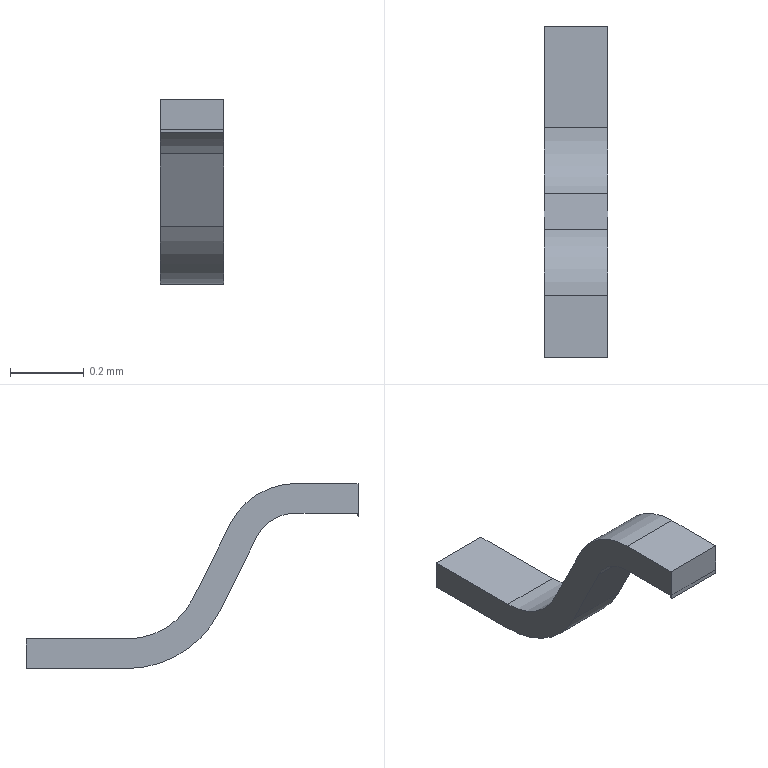Part | STEP file | RJ-USIO-V1_2-220411_5 | 1 solid | 15 faces | box 0.1708 x 0.8974 x 0.5 mm | volume 0.01511 mm3 | plane 11 | cylinder 4 | commonest cylinder face diameters 0.4 x2 0.24 x1 0.56 x1
STEP:
#1=CARTESIAN_POINT('',(0.,0.,0.));
#2=DIRECTION('',(0.,0.,1.));
#3=DIRECTION('',(1.,0.,0.));
#4=AXIS2_PLACEMENT_3D('',#1,#2,#3);
#5=CARTESIAN_POINT('',(46.936,55.937,0.3886));
#6=VERTEX_POINT('',#5);
#7=CARTESIAN_POINT('',(46.765,55.937,0.3886));
#8=VERTEX_POINT('',#7);
#9=CARTESIAN_POINT('',(46.936,55.937,0.3886));
#10=DIRECTION('',(-1.,0.,0.));
#11=VECTOR('',#10,1.);
#12=LINE('',#9,#11);
#13=CARTESIAN_POINT('',(44.809,55.758,0.3));
#14=DIRECTION('',(1.,0.,0.));
#15=DIRECTION('',(0.,0.,1.));
#16=AXIS2_PLACEMENT_3D('',#13,#14,#15);
#17=CYLINDRICAL_SURFACE('',#16,0.2);
#18=CARTESIAN_POINT('',(5.172,2.127));
#19=DIRECTION('',(0.,-1.));
#20=VECTOR('',#19,1.);
#21=LINE('',#18,#20);
#22=(GEOMETRIC_REPRESENTATION_CONTEXT(2)PARAMETRIC_REPRESENTATION_CONTEXT()REPRESENTATION_CONTEXT('',''));
#23=DEFINITIONAL_REPRESENTATION('',(#21),#22);
#24=PCURVE('',#17,#23);
#25=CARTESIAN_POINT('',(44.809,56.035,0.1914));
#26=DIRECTION('',(0.,-0.8964,-0.4432));
#27=DIRECTION('',(0.,-0.4432,0.8964));
#28=AXIS2_PLACEMENT_3D('',#25,#26,#27);
#29=PLANE('',#28);
#30=CARTESIAN_POINT('',(0.2201,-2.127));
#31=DIRECTION('',(0.,1.));
#32=VECTOR('',#31,1.);
#33=LINE('',#30,#32);
#34=(GEOMETRIC_REPRESENTATION_CONTEXT(2)PARAMETRIC_REPRESENTATION_CONTEXT()REPRESENTATION_CONTEXT('',''));
#35=DEFINITIONAL_REPRESENTATION('',(#33),#34);
#36=PCURVE('',#29,#35);
#37=SURFACE_CURVE('',#12,(#24,#36),.PCURVE_S1.);
#38=EDGE_CURVE('',#6,#8,#37,.T.);
#39=ORIENTED_EDGE('',*,*,#38,.T.);
#40=CARTESIAN_POINT('',(46.765,55.758,0.5));
#41=VERTEX_POINT('',#40);
#42=CARTESIAN_POINT('',(46.765,55.758,0.3));
#43=DIRECTION('',(-1.,0.,0.));
#44=DIRECTION('',(0.,0.,1.));
#45=AXIS2_PLACEMENT_3D('',#42,#43,#44);
#46=CIRCLE('',#45,0.2);
#47=CARTESIAN_POINT('',(6.283,1.956));
#48=DIRECTION('',(-1.,0.));
#49=VECTOR('',#48,1.);
#50=LINE('',#47,#49);
#51=(GEOMETRIC_REPRESENTATION_CONTEXT(2)PARAMETRIC_REPRESENTATION_CONTEXT()REPRESENTATION_CONTEXT('',''));
#52=DEFINITIONAL_REPRESENTATION('',(#50),#51);
#53=PCURVE('',#17,#52);
#54=CARTESIAN_POINT('',(46.765,56.487,0.5));
#55=DIRECTION('',(-1.,0.,0.));
#56=DIRECTION('',(0.,0.,-1.));
#57=AXIS2_PLACEMENT_3D('',#54,#55,#56);
#58=PLANE('',#57);
#59=CARTESIAN_POINT('',(0.2,0.7295));
#60=DIRECTION('',(-1.,0.));
#61=AXIS2_PLACEMENT_2D('',#59,#60);
#62=CIRCLE('',#61,0.2);
#63=(GEOMETRIC_REPRESENTATION_CONTEXT(2)PARAMETRIC_REPRESENTATION_CONTEXT()REPRESENTATION_CONTEXT('',''));
#64=DEFINITIONAL_REPRESENTATION('',(#62),#63);
#65=PCURVE('',#58,#64);
#66=SURFACE_CURVE('',#46,(#53,#65),.PCURVE_S1.);
#67=EDGE_CURVE('',#41,#8,#66,.T.);
#68=ORIENTED_EDGE('',*,*,#67,.F.);
#69=CARTESIAN_POINT('',(46.936,55.758,0.5));
#70=VERTEX_POINT('',#69);
#71=CARTESIAN_POINT('',(46.765,55.758,0.5));
#72=DIRECTION('',(1.,0.,0.));
#73=VECTOR('',#72,1.);
#74=LINE('',#71,#73);
#75=CARTESIAN_POINT('',(6.283,1.956));
#76=DIRECTION('',(0.,1.));
#77=VECTOR('',#76,1.);
#78=LINE('',#75,#77);
#79=(GEOMETRIC_REPRESENTATION_CONTEXT(2)PARAMETRIC_REPRESENTATION_CONTEXT()REPRESENTATION_CONTEXT('',''));
#80=DEFINITIONAL_REPRESENTATION('',(#78),#79);
#81=PCURVE('',#17,#80);
#82=CARTESIAN_POINT('',(46.936,55.59,0.5));
#83=DIRECTION('',(0.,0.,-1.));
#84=DIRECTION('',(1.,0.,0.));
#85=AXIS2_PLACEMENT_3D('',#82,#83,#84);
#86=PLANE('',#85);
#87=CARTESIAN_POINT('',(-0.1708,-0.1678));
#88=DIRECTION('',(1.,0.));
#89=VECTOR('',#88,1.);
#90=LINE('',#87,#89);
#91=(GEOMETRIC_REPRESENTATION_CONTEXT(2)PARAMETRIC_REPRESENTATION_CONTEXT()REPRESENTATION_CONTEXT('',''));
#92=DEFINITIONAL_REPRESENTATION('',(#90),#91);
#93=PCURVE('',#86,#92);
#94=SURFACE_CURVE('',#74,(#81,#93),.PCURVE_S1.);
#95=EDGE_CURVE('',#41,#70,#94,.T.);
#96=ORIENTED_EDGE('',*,*,#95,.T.);
#97=CARTESIAN_POINT('',(46.936,55.758,0.3));
#98=DIRECTION('',(1.,0.,0.));
#99=DIRECTION('',(0.,0.8964,0.4432));
#100=AXIS2_PLACEMENT_3D('',#97,#98,#99);
#101=CIRCLE('',#100,0.2);
#102=CARTESIAN_POINT('',(5.172,2.127));
#103=DIRECTION('',(1.,0.));
#104=VECTOR('',#103,1.);
#105=LINE('',#102,#104);
#106=(GEOMETRIC_REPRESENTATION_CONTEXT(2)PARAMETRIC_REPRESENTATION_CONTEXT()REPRESENTATION_CONTEXT('',''));
#107=DEFINITIONAL_REPRESENTATION('',(#105),#106);
#108=PCURVE('',#17,#107);
#109=CARTESIAN_POINT('',(46.936,56.487,0.5));
#110=DIRECTION('',(1.,0.,0.));
#111=DIRECTION('',(0.,0.,1.));
#112=AXIS2_PLACEMENT_3D('',#109,#110,#111);
#113=PLANE('',#112);
#114=CARTESIAN_POINT('',(-0.2,0.7295));
#115=DIRECTION('',(0.4432,-0.8964));
#116=AXIS2_PLACEMENT_2D('',#114,#115);
#117=CIRCLE('',#116,0.2);
#118=(GEOMETRIC_REPRESENTATION_CONTEXT(2)PARAMETRIC_REPRESENTATION_CONTEXT()REPRESENTATION_CONTEXT('',''));
#119=DEFINITIONAL_REPRESENTATION('',(#117),#118);
#120=PCURVE('',#113,#119);
#121=SURFACE_CURVE('',#101,(#108,#120),.PCURVE_S1.);
#122=EDGE_CURVE('',#6,#70,#121,.T.);
#123=ORIENTED_EDGE('',*,*,#122,.F.);
#124=EDGE_LOOP('',(#39,#68,#96,#123));
#125=FACE_BOUND('',#124,.T.);
#126=ADVANCED_FACE('',(#125),#17,.T.);
#127=CARTESIAN_POINT('',(46.936,56.487,0.08));
#128=VERTEX_POINT('',#127);
#129=CARTESIAN_POINT('',(46.936,56.214,0.08));
#130=VERTEX_POINT('',#129);
#131=CARTESIAN_POINT('',(46.936,56.487,0.08));
#132=DIRECTION('',(0.,-1.,0.));
#133=VECTOR('',#132,1.);
#134=LINE('',#131,#133);
#135=CARTESIAN_POINT('',(-0.42,0.));
#136=DIRECTION('',(0.,1.));
#137=VECTOR('',#136,1.);
#138=LINE('',#135,#137);
#139=(GEOMETRIC_REPRESENTATION_CONTEXT(2)PARAMETRIC_REPRESENTATION_CONTEXT()REPRESENTATION_CONTEXT('',''));
#140=DEFINITIONAL_REPRESENTATION('',(#138),#139);
#141=PCURVE('',#113,#140);
#142=CARTESIAN_POINT('',(44.809,56.491,0.08));
#143=DIRECTION('',(0.,0.,-1.));
#144=DIRECTION('',(1.,0.,0.));
#145=AXIS2_PLACEMENT_3D('',#142,#143,#144);
#146=PLANE('',#145);
#147=CARTESIAN_POINT('',(2.127,0.003694));
#148=DIRECTION('',(0.,1.));
#149=VECTOR('',#148,1.);
#150=LINE('',#147,#149);
#151=(GEOMETRIC_REPRESENTATION_CONTEXT(2)PARAMETRIC_REPRESENTATION_CONTEXT()REPRESENTATION_CONTEXT('',''));
#152=DEFINITIONAL_REPRESENTATION('',(#150),#151);
#153=PCURVE('',#146,#152);
#154=SURFACE_CURVE('',#134,(#141,#153),.PCURVE_S1.);
#155=EDGE_CURVE('',#128,#130,#154,.T.);
#156=ORIENTED_EDGE('',*,*,#155,.F.);
#157=CARTESIAN_POINT('',(46.936,56.487,0.));
#158=VERTEX_POINT('',#157);
#159=CARTESIAN_POINT('',(46.936,56.487,0.));
#160=DIRECTION('',(0.,0.,1.));
#161=VECTOR('',#160,1.);
#162=LINE('',#159,#161);
#163=CARTESIAN_POINT('',(-0.5,0.));
#164=DIRECTION('',(1.,0.));
#165=VECTOR('',#164,1.);
#166=LINE('',#163,#165);
#167=(GEOMETRIC_REPRESENTATION_CONTEXT(2)PARAMETRIC_REPRESENTATION_CONTEXT()REPRESENTATION_CONTEXT('',''));
#168=DEFINITIONAL_REPRESENTATION('',(#166),#167);
#169=PCURVE('',#113,#168);
#170=CARTESIAN_POINT('',(46.936,56.487,0.5));
#171=DIRECTION('',(0.,1.,0.));
#172=DIRECTION('',(0.,0.,-1.));
#173=AXIS2_PLACEMENT_3D('',#170,#171,#172);
#174=PLANE('',#173);
#175=CARTESIAN_POINT('',(0.5,0.));
#176=DIRECTION('',(-1.,0.));
#177=VECTOR('',#176,1.);
#178=LINE('',#175,#177);
#179=(GEOMETRIC_REPRESENTATION_CONTEXT(2)PARAMETRIC_REPRESENTATION_CONTEXT()REPRESENTATION_CONTEXT('',''));
#180=DEFINITIONAL_REPRESENTATION('',(#178),#179);
#181=PCURVE('',#174,#180);
#182=SURFACE_CURVE('',#162,(#169,#181),.PCURVE_S1.);
#183=EDGE_CURVE('',#158,#128,#182,.T.);
#184=ORIENTED_EDGE('',*,*,#183,.F.);
#185=CARTESIAN_POINT('',(46.936,56.214,0.));
#186=VERTEX_POINT('',#185);
#187=CARTESIAN_POINT('',(46.936,56.214,0.));
#188=DIRECTION('',(0.,1.,0.));
#189=VECTOR('',#188,1.);
#190=LINE('',#187,#189);
#191=CARTESIAN_POINT('',(-0.5,0.2734));
#192=DIRECTION('',(0.,-1.));
#193=VECTOR('',#192,1.);
#194=LINE('',#191,#193);
#195=(GEOMETRIC_REPRESENTATION_CONTEXT(2)PARAMETRIC_REPRESENTATION_CONTEXT()REPRESENTATION_CONTEXT('',''));
#196=DEFINITIONAL_REPRESENTATION('',(#194),#195);
#197=PCURVE('',#113,#196);
#198=CARTESIAN_POINT('',(46.936,55.59,0.));
#199=DIRECTION('',(0.,0.,-1.));
#200=DIRECTION('',(1.,0.,0.));
#201=AXIS2_PLACEMENT_3D('',#198,#199,#200);
#202=PLANE('',#201);
#203=CARTESIAN_POINT('',(0.,-0.6239));
#204=DIRECTION('',(0.,-1.));
#205=VECTOR('',#204,1.);
#206=LINE('',#203,#205);
#207=(GEOMETRIC_REPRESENTATION_CONTEXT(2)PARAMETRIC_REPRESENTATION_CONTEXT()REPRESENTATION_CONTEXT('',''));
#208=DEFINITIONAL_REPRESENTATION('',(#206),#207);
#209=PCURVE('',#202,#208);
#210=SURFACE_CURVE('',#190,(#197,#209),.PCURVE_S1.);
#211=EDGE_CURVE('',#186,#158,#210,.T.);
#212=ORIENTED_EDGE('',*,*,#211,.F.);
#213=CARTESIAN_POINT('',(46.936,55.963,0.1559));
#214=VERTEX_POINT('',#213);
#215=CARTESIAN_POINT('',(46.936,56.214,0.28));
#216=DIRECTION('',(1.,0.,0.));
#217=DIRECTION('',(0.,-0.8964,-0.4432));
#218=AXIS2_PLACEMENT_3D('',#215,#216,#217);
#219=CIRCLE('',#218,0.28);
#220=CARTESIAN_POINT('',(-0.22,0.2734));
#221=DIRECTION('',(-0.4432,0.8964));
#222=AXIS2_PLACEMENT_2D('',#220,#221);
#223=CIRCLE('',#222,0.28);
#224=(GEOMETRIC_REPRESENTATION_CONTEXT(2)PARAMETRIC_REPRESENTATION_CONTEXT()REPRESENTATION_CONTEXT('',''));
#225=DEFINITIONAL_REPRESENTATION('',(#223),#224);
#226=PCURVE('',#113,#225);
#227=CARTESIAN_POINT('',(44.809,56.214,0.28));
#228=DIRECTION('',(1.,0.,0.));
#229=DIRECTION('',(0.,0.,1.));
#230=AXIS2_PLACEMENT_3D('',#227,#228,#229);
#231=CYLINDRICAL_SURFACE('',#230,0.28);
#232=CARTESIAN_POINT('',(2.03,2.127));
#233=DIRECTION('',(1.,0.));
#234=VECTOR('',#233,1.);
#235=LINE('',#232,#234);
#236=(GEOMETRIC_REPRESENTATION_CONTEXT(2)PARAMETRIC_REPRESENTATION_CONTEXT()REPRESENTATION_CONTEXT('',''));
#237=DEFINITIONAL_REPRESENTATION('',(#235),#236);
#238=PCURVE('',#231,#237);
#239=SURFACE_CURVE('',#219,(#226,#238),.PCURVE_S1.);
#240=EDGE_CURVE('',#214,#186,#239,.T.);
#241=ORIENTED_EDGE('',*,*,#240,.F.);
#242=CARTESIAN_POINT('',(46.936,55.865,0.3532));
#243=VERTEX_POINT('',#242);
#244=CARTESIAN_POINT('',(46.936,55.865,0.3532));
#245=DIRECTION('',(0.,0.4432,-0.8964));
#246=VECTOR('',#245,1.);
#247=LINE('',#244,#246);
#248=CARTESIAN_POINT('',(-0.1468,0.622));
#249=DIRECTION('',(-0.8964,-0.4432));
#250=VECTOR('',#249,1.);
#251=LINE('',#248,#250);
#252=(GEOMETRIC_REPRESENTATION_CONTEXT(2)PARAMETRIC_REPRESENTATION_CONTEXT()REPRESENTATION_CONTEXT('',''));
#253=DEFINITIONAL_REPRESENTATION('',(#251),#252);
#254=PCURVE('',#113,#253);
#255=CARTESIAN_POINT('',(44.809,55.963,0.1559));
#256=DIRECTION('',(0.,0.8964,0.4432));
#257=DIRECTION('',(0.,0.4432,-0.8964));
#258=AXIS2_PLACEMENT_3D('',#255,#256,#257);
#259=PLANE('',#258);
#260=CARTESIAN_POINT('',(-0.2201,-2.127));
#261=DIRECTION('',(1.,0.));
#262=VECTOR('',#261,1.);
#263=LINE('',#260,#262);
#264=(GEOMETRIC_REPRESENTATION_CONTEXT(2)PARAMETRIC_REPRESENTATION_CONTEXT()REPRESENTATION_CONTEXT('',''));
#265=DEFINITIONAL_REPRESENTATION('',(#263),#264);
#266=PCURVE('',#259,#265);
#267=SURFACE_CURVE('',#247,(#254,#266),.PCURVE_S1.);
#268=EDGE_CURVE('',#243,#214,#267,.T.);
#269=ORIENTED_EDGE('',*,*,#268,.F.);
#270=CARTESIAN_POINT('',(46.936,55.758,0.42));
#271=VERTEX_POINT('',#270);
#272=CARTESIAN_POINT('',(46.936,55.758,0.3));
#273=DIRECTION('',(-1.,0.,0.));
#274=DIRECTION('',(0.,0.,1.));
#275=AXIS2_PLACEMENT_3D('',#272,#273,#274);
#276=CIRCLE('',#275,0.12);
#277=CARTESIAN_POINT('',(-0.08,0.7295));
#278=CARTESIAN_POINT('',(-0.08,0.5217));
#279=CARTESIAN_POINT('',(-0.26,0.6256));
#280=CARTESIAN_POINT('',(-0.44,0.7295));
#281=CARTESIAN_POINT('',(-0.26,0.8335));
#282=CARTESIAN_POINT('',(-0.08,0.9374));
#283=CARTESIAN_POINT('',(-0.08,0.7295));
#284=(BOUNDED_CURVE()B_SPLINE_CURVE(2,(#277,#278,#279,#280,#281,#282,#283),.UNSPECIFIED.,.T.,.F.)B_SPLINE_CURVE_WITH_KNOTS((1,2,2,2,2,1),(-2.094,0.,2.094,4.189,6.283,8.378),.UNSPECIFIED.)CURVE()GEOMETRIC_REPRESENTATION_ITEM()RATIONAL_B_SPLINE_CURVE((1.,0.5,1.,0.5,1.,0.5,1.))REPRESENTATION_ITEM(''));
#285=(GEOMETRIC_REPRESENTATION_CONTEXT(2)PARAMETRIC_REPRESENTATION_CONTEXT()REPRESENTATION_CONTEXT('',''));
#286=DEFINITIONAL_REPRESENTATION('',(#284),#285);
#287=PCURVE('',#113,#286);
#288=CARTESIAN_POINT('',(44.809,55.758,0.3));
#289=DIRECTION('',(1.,0.,0.));
#290=DIRECTION('',(0.,0.,1.));
#291=AXIS2_PLACEMENT_3D('',#288,#289,#290);
#292=CYLINDRICAL_SURFACE('',#291,0.12);
#293=CARTESIAN_POINT('',(6.283,2.127));
#294=DIRECTION('',(-1.,0.));
#295=VECTOR('',#294,1.);
#296=LINE('',#293,#295);
#297=(GEOMETRIC_REPRESENTATION_CONTEXT(2)PARAMETRIC_REPRESENTATION_CONTEXT()REPRESENTATION_CONTEXT('',''));
#298=DEFINITIONAL_REPRESENTATION('',(#296),#297);
#299=PCURVE('',#292,#298);
#300=SURFACE_CURVE('',#276,(#287,#299),.PCURVE_S1.);
#301=EDGE_CURVE('',#271,#243,#300,.T.);
#302=ORIENTED_EDGE('',*,*,#301,.F.);
#303=CARTESIAN_POINT('',(46.936,55.591,0.42));
#304=VERTEX_POINT('',#303);
#305=CARTESIAN_POINT('',(46.936,55.591,0.42));
#306=DIRECTION('',(0.,1.,0.));
#307=VECTOR('',#306,1.);
#308=LINE('',#305,#307);
#309=CARTESIAN_POINT('',(-0.08,0.8961));
#310=DIRECTION('',(0.,-1.));
#311=VECTOR('',#310,1.);
#312=LINE('',#309,#311);
#313=(GEOMETRIC_REPRESENTATION_CONTEXT(2)PARAMETRIC_REPRESENTATION_CONTEXT()REPRESENTATION_CONTEXT('',''));
#314=DEFINITIONAL_REPRESENTATION('',(#312),#313);
#315=PCURVE('',#113,#314);
#316=CARTESIAN_POINT('',(44.809,55.758,0.42));
#317=DIRECTION('',(0.,0.,1.));
#318=DIRECTION('',(-1.,0.,0.));
#319=AXIS2_PLACEMENT_3D('',#316,#317,#318);
#320=PLANE('',#319);
#321=CARTESIAN_POINT('',(-2.127,0.1665));
#322=DIRECTION('',(0.,-1.));
#323=VECTOR('',#322,1.);
#324=LINE('',#321,#323);
#325=(GEOMETRIC_REPRESENTATION_CONTEXT(2)PARAMETRIC_REPRESENTATION_CONTEXT()REPRESENTATION_CONTEXT('',''));
#326=DEFINITIONAL_REPRESENTATION('',(#324),#325);
#327=PCURVE('',#320,#326);
#328=SURFACE_CURVE('',#308,(#315,#327),.PCURVE_S1.);
#329=EDGE_CURVE('',#304,#271,#328,.T.);
#330=ORIENTED_EDGE('',*,*,#329,.F.);
#331=CARTESIAN_POINT('',(46.936,55.59,0.4096));
#332=VERTEX_POINT('',#331);
#333=CARTESIAN_POINT('',(46.936,55.59,0.4096));
#334=DIRECTION('',(0.,0.1219,0.9925));
#335=VECTOR('',#334,1.);
#336=LINE('',#333,#335);
#337=CARTESIAN_POINT('',(-0.09045,0.8974));
#338=DIRECTION('',(0.9925,-0.1219));
#339=VECTOR('',#338,1.);
#340=LINE('',#337,#339);
#341=(GEOMETRIC_REPRESENTATION_CONTEXT(2)PARAMETRIC_REPRESENTATION_CONTEXT()REPRESENTATION_CONTEXT('',''));
#342=DEFINITIONAL_REPRESENTATION('',(#340),#341);
#343=PCURVE('',#113,#342);
#344=CARTESIAN_POINT('',(44.809,55.591,0.42));
#345=DIRECTION('',(0.,-0.9925,0.1219));
#346=DIRECTION('',(0.,0.1219,0.9925));
#347=AXIS2_PLACEMENT_3D('',#344,#345,#346);
#348=PLANE('',#347);
#349=CARTESIAN_POINT('',(-0.01053,-2.127));
#350=DIRECTION('',(1.,0.));
#351=VECTOR('',#350,1.);
#352=LINE('',#349,#351);
#353=(GEOMETRIC_REPRESENTATION_CONTEXT(2)PARAMETRIC_REPRESENTATION_CONTEXT()REPRESENTATION_CONTEXT('',''));
#354=DEFINITIONAL_REPRESENTATION('',(#352),#353);
#355=PCURVE('',#348,#354);
#356=SURFACE_CURVE('',#336,(#343,#355),.PCURVE_S1.);
#357=EDGE_CURVE('',#332,#304,#356,.T.);
#358=ORIENTED_EDGE('',*,*,#357,.F.);
#359=CARTESIAN_POINT('',(46.936,55.59,0.5));
#360=VERTEX_POINT('',#359);
#361=CARTESIAN_POINT('',(46.936,55.59,0.4096));
#362=DIRECTION('',(0.,0.,1.));
#363=VECTOR('',#362,1.);
#364=LINE('',#361,#363);
#365=CARTESIAN_POINT('',(-0.09045,0.8974));
#366=DIRECTION('',(1.,0.));
#367=VECTOR('',#366,1.);
#368=LINE('',#365,#367);
#369=(GEOMETRIC_REPRESENTATION_CONTEXT(2)PARAMETRIC_REPRESENTATION_CONTEXT()REPRESENTATION_CONTEXT('',''));
#370=DEFINITIONAL_REPRESENTATION('',(#368),#369);
#371=PCURVE('',#113,#370);
#372=CARTESIAN_POINT('',(46.936,55.59,0.5));
#373=DIRECTION('',(0.,-1.,0.));
#374=DIRECTION('',(0.,0.,1.));
#375=AXIS2_PLACEMENT_3D('',#372,#373,#374);
#376=PLANE('',#375);
#377=CARTESIAN_POINT('',(-0.09045,0.));
#378=DIRECTION('',(1.,0.));
#379=VECTOR('',#378,1.);
#380=LINE('',#377,#379);
#381=(GEOMETRIC_REPRESENTATION_CONTEXT(2)PARAMETRIC_REPRESENTATION_CONTEXT()REPRESENTATION_CONTEXT('',''));
#382=DEFINITIONAL_REPRESENTATION('',(#380),#381);
#383=PCURVE('',#376,#382);
#384=SURFACE_CURVE('',#364,(#371,#383),.PCURVE_S1.);
#385=EDGE_CURVE('',#332,#360,#384,.T.);
#386=ORIENTED_EDGE('',*,*,#385,.T.);
#387=CARTESIAN_POINT('',(46.936,55.59,0.5));
#388=DIRECTION('',(0.,1.,0.));
#389=VECTOR('',#388,1.);
#390=LINE('',#387,#389);
#391=CARTESIAN_POINT('',(0.,0.8974));
#392=DIRECTION('',(0.,-1.));
#393=VECTOR('',#392,1.);
#394=LINE('',#391,#393);
#395=(GEOMETRIC_REPRESENTATION_CONTEXT(2)PARAMETRIC_REPRESENTATION_CONTEXT()REPRESENTATION_CONTEXT('',''));
#396=DEFINITIONAL_REPRESENTATION('',(#394),#395);
#397=PCURVE('',#113,#396);
#398=CARTESIAN_POINT('',(0.,0.));
#399=DIRECTION('',(0.,-1.));
#400=VECTOR('',#399,1.);
#401=LINE('',#398,#400);
#402=(GEOMETRIC_REPRESENTATION_CONTEXT(2)PARAMETRIC_REPRESENTATION_CONTEXT()REPRESENTATION_CONTEXT('',''));
#403=DEFINITIONAL_REPRESENTATION('',(#401),#402);
#404=PCURVE('',#86,#403);
#405=SURFACE_CURVE('',#390,(#397,#404),.PCURVE_S1.);
#406=EDGE_CURVE('',#360,#70,#405,.T.);
#407=ORIENTED_EDGE('',*,*,#406,.T.);
#408=ORIENTED_EDGE('',*,*,#122,.F.);
#409=CARTESIAN_POINT('',(46.936,56.035,0.1914));
#410=VERTEX_POINT('',#409);
#411=CARTESIAN_POINT('',(46.936,56.035,0.1914));
#412=DIRECTION('',(0.,-0.4432,0.8964));
#413=VECTOR('',#412,1.);
#414=LINE('',#411,#413);
#415=CARTESIAN_POINT('',(-0.3086,0.4527));
#416=DIRECTION('',(0.8964,0.4432));
#417=VECTOR('',#416,1.);
#418=LINE('',#415,#417);
#419=(GEOMETRIC_REPRESENTATION_CONTEXT(2)PARAMETRIC_REPRESENTATION_CONTEXT()REPRESENTATION_CONTEXT('',''));
#420=DEFINITIONAL_REPRESENTATION('',(#418),#419);
#421=PCURVE('',#113,#420);
#422=CARTESIAN_POINT('',(0.,-2.127));
#423=DIRECTION('',(1.,0.));
#424=VECTOR('',#423,1.);
#425=LINE('',#422,#424);
#426=(GEOMETRIC_REPRESENTATION_CONTEXT(2)PARAMETRIC_REPRESENTATION_CONTEXT()REPRESENTATION_CONTEXT('',''));
#427=DEFINITIONAL_REPRESENTATION('',(#425),#426);
#428=PCURVE('',#29,#427);
#429=SURFACE_CURVE('',#414,(#421,#428),.PCURVE_S1.);
#430=EDGE_CURVE('',#410,#6,#429,.T.);
#431=ORIENTED_EDGE('',*,*,#430,.F.);
#432=CARTESIAN_POINT('',(46.936,56.214,0.28));
#433=DIRECTION('',(-1.,0.,0.));
#434=DIRECTION('',(0.,0.,-1.));
#435=AXIS2_PLACEMENT_3D('',#432,#433,#434);
#436=CIRCLE('',#435,0.2);
#437=CARTESIAN_POINT('',(-0.42,0.2734));
#438=CARTESIAN_POINT('',(-0.42,0.6198));
#439=CARTESIAN_POINT('',(-0.12,0.4466));
#440=CARTESIAN_POINT('',(0.18,0.2734));
#441=CARTESIAN_POINT('',(-0.12,0.1002));
#442=CARTESIAN_POINT('',(-0.42,-0.07299));
#443=CARTESIAN_POINT('',(-0.42,0.2734));
#444=(BOUNDED_CURVE()B_SPLINE_CURVE(2,(#437,#438,#439,#440,#441,#442,#443),.UNSPECIFIED.,.T.,.F.)B_SPLINE_CURVE_WITH_KNOTS((1,2,2,2,2,1),(-2.094,0.,2.094,4.189,6.283,8.378),.UNSPECIFIED.)CURVE()GEOMETRIC_REPRESENTATION_ITEM()RATIONAL_B_SPLINE_CURVE((1.,0.5,1.,0.5,1.,0.5,1.))REPRESENTATION_ITEM(''));
#445=(GEOMETRIC_REPRESENTATION_CONTEXT(2)PARAMETRIC_REPRESENTATION_CONTEXT()REPRESENTATION_CONTEXT('',''));
#446=DEFINITIONAL_REPRESENTATION('',(#444),#445);
#447=PCURVE('',#113,#446);
#448=CARTESIAN_POINT('',(44.809,56.214,0.28));
#449=DIRECTION('',(1.,0.,0.));
#450=DIRECTION('',(0.,0.,1.));
#451=AXIS2_PLACEMENT_3D('',#448,#449,#450);
#452=CYLINDRICAL_SURFACE('',#451,0.2);
#453=CARTESIAN_POINT('',(3.142,2.127));
#454=DIRECTION('',(-1.,0.));
#455=VECTOR('',#454,1.);
#456=LINE('',#453,#455);
#457=(GEOMETRIC_REPRESENTATION_CONTEXT(2)PARAMETRIC_REPRESENTATION_CONTEXT()REPRESENTATION_CONTEXT('',''));
#458=DEFINITIONAL_REPRESENTATION('',(#456),#457);
#459=PCURVE('',#452,#458);
#460=SURFACE_CURVE('',#436,(#447,#459),.PCURVE_S1.);
#461=EDGE_CURVE('',#130,#410,#460,.T.);
#462=ORIENTED_EDGE('',*,*,#461,.F.);
#463=EDGE_LOOP('',(#156,#184,#212,#241,#269,#302,#330,#358,#386,#407,#408,#431,#462));
#464=FACE_BOUND('',#463,.F.);
#465=ADVANCED_FACE('',(#464),#113,.T.);
#466=ORIENTED_EDGE('',*,*,#155,.T.);
#467=CARTESIAN_POINT('',(46.765,56.214,0.08));
#468=VERTEX_POINT('',#467);
#469=CARTESIAN_POINT('',(46.936,56.214,0.08));
#470=DIRECTION('',(-1.,0.,0.));
#471=VECTOR('',#470,1.);
#472=LINE('',#469,#471);
#473=CARTESIAN_POINT('',(2.127,0.2771));
#474=DIRECTION('',(-1.,0.));
#475=VECTOR('',#474,1.);
#476=LINE('',#473,#475);
#477=(GEOMETRIC_REPRESENTATION_CONTEXT(2)PARAMETRIC_REPRESENTATION_CONTEXT()REPRESENTATION_CONTEXT('',''));
#478=DEFINITIONAL_REPRESENTATION('',(#476),#477);
#479=PCURVE('',#146,#478);
#480=CARTESIAN_POINT('',(3.142,2.127));
#481=DIRECTION('',(0.,-1.));
#482=VECTOR('',#481,1.);
#483=LINE('',#480,#482);
#484=(GEOMETRIC_REPRESENTATION_CONTEXT(2)PARAMETRIC_REPRESENTATION_CONTEXT()REPRESENTATION_CONTEXT('',''));
#485=DEFINITIONAL_REPRESENTATION('',(#483),#484);
#486=PCURVE('',#452,#485);
#487=SURFACE_CURVE('',#472,(#479,#486),.PCURVE_S1.);
#488=EDGE_CURVE('',#130,#468,#487,.T.);
#489=ORIENTED_EDGE('',*,*,#488,.T.);
#490=CARTESIAN_POINT('',(46.765,56.487,0.08));
#491=VERTEX_POINT('',#490);
#492=CARTESIAN_POINT('',(46.765,56.214,0.08));
#493=DIRECTION('',(0.,1.,0.));
#494=VECTOR('',#493,1.);
#495=LINE('',#492,#494);
#496=CARTESIAN_POINT('',(1.956,0.2771));
#497=DIRECTION('',(0.,-1.));
#498=VECTOR('',#497,1.);
#499=LINE('',#496,#498);
#500=(GEOMETRIC_REPRESENTATION_CONTEXT(2)PARAMETRIC_REPRESENTATION_CONTEXT()REPRESENTATION_CONTEXT('',''));
#501=DEFINITIONAL_REPRESENTATION('',(#499),#500);
#502=PCURVE('',#146,#501);
#503=CARTESIAN_POINT('',(0.42,0.2734));
#504=DIRECTION('',(0.,-1.));
#505=VECTOR('',#504,1.);
#506=LINE('',#503,#505);
#507=(GEOMETRIC_REPRESENTATION_CONTEXT(2)PARAMETRIC_REPRESENTATION_CONTEXT()REPRESENTATION_CONTEXT('',''));
#508=DEFINITIONAL_REPRESENTATION('',(#506),#507);
#509=PCURVE('',#58,#508);
#510=SURFACE_CURVE('',#495,(#502,#509),.PCURVE_S1.);
#511=EDGE_CURVE('',#468,#491,#510,.T.);
#512=ORIENTED_EDGE('',*,*,#511,.T.);
#513=CARTESIAN_POINT('',(46.765,56.487,0.08));
#514=DIRECTION('',(1.,0.,0.));
#515=VECTOR('',#514,1.);
#516=LINE('',#513,#515);
#517=CARTESIAN_POINT('',(1.956,0.003694));
#518=DIRECTION('',(1.,0.));
#519=VECTOR('',#518,1.);
#520=LINE('',#517,#519);
#521=(GEOMETRIC_REPRESENTATION_CONTEXT(2)PARAMETRIC_REPRESENTATION_CONTEXT()REPRESENTATION_CONTEXT('',''));
#522=DEFINITIONAL_REPRESENTATION('',(#520),#521);
#523=PCURVE('',#146,#522);
#524=CARTESIAN_POINT('',(0.42,0.1708));
#525=DIRECTION('',(0.,-1.));
#526=VECTOR('',#525,1.);
#527=LINE('',#524,#526);
#528=(GEOMETRIC_REPRESENTATION_CONTEXT(2)PARAMETRIC_REPRESENTATION_CONTEXT()REPRESENTATION_CONTEXT('',''));
#529=DEFINITIONAL_REPRESENTATION('',(#527),#528);
#530=PCURVE('',#174,#529);
#531=SURFACE_CURVE('',#516,(#523,#530),.PCURVE_S1.);
#532=EDGE_CURVE('',#491,#128,#531,.T.);
#533=ORIENTED_EDGE('',*,*,#532,.T.);
#534=EDGE_LOOP('',(#466,#489,#512,#533));
#535=FACE_BOUND('',#534,.F.);
#536=ADVANCED_FACE('',(#535),#146,.F.);
#537=ORIENTED_EDGE('',*,*,#461,.T.);
#538=CARTESIAN_POINT('',(46.765,56.035,0.1914));
#539=VERTEX_POINT('',#538);
#540=CARTESIAN_POINT('',(46.765,56.035,0.1914));
#541=DIRECTION('',(1.,0.,0.));
#542=VECTOR('',#541,1.);
#543=LINE('',#540,#542);
#544=CARTESIAN_POINT('',(2.03,1.956));
#545=DIRECTION('',(0.,1.));
#546=VECTOR('',#545,1.);
#547=LINE('',#544,#546);
#548=(GEOMETRIC_REPRESENTATION_CONTEXT(2)PARAMETRIC_REPRESENTATION_CONTEXT()REPRESENTATION_CONTEXT('',''));
#549=DEFINITIONAL_REPRESENTATION('',(#547),#548);
#550=PCURVE('',#452,#549);
#551=CARTESIAN_POINT('',(0.,-1.956));
#552=DIRECTION('',(0.,-1.));
#553=VECTOR('',#552,1.);
#554=LINE('',#551,#553);
#555=(GEOMETRIC_REPRESENTATION_CONTEXT(2)PARAMETRIC_REPRESENTATION_CONTEXT()REPRESENTATION_CONTEXT('',''));
#556=DEFINITIONAL_REPRESENTATION('',(#554),#555);
#557=PCURVE('',#29,#556);
#558=SURFACE_CURVE('',#543,(#550,#557),.PCURVE_S1.);
#559=EDGE_CURVE('',#539,#410,#558,.T.);
#560=ORIENTED_EDGE('',*,*,#559,.F.);
#561=CARTESIAN_POINT('',(46.765,56.214,0.28));
#562=DIRECTION('',(1.,0.,0.));
#563=DIRECTION('',(0.,-0.8964,-0.4432));
#564=AXIS2_PLACEMENT_3D('',#561,#562,#563);
#565=CIRCLE('',#564,0.2);
#566=CARTESIAN_POINT('',(2.03,1.956));
#567=DIRECTION('',(1.,0.));
#568=VECTOR('',#567,1.);
#569=LINE('',#566,#568);
#570=(GEOMETRIC_REPRESENTATION_CONTEXT(2)PARAMETRIC_REPRESENTATION_CONTEXT()REPRESENTATION_CONTEXT('',''));
#571=DEFINITIONAL_REPRESENTATION('',(#569),#570);
#572=PCURVE('',#452,#571);
#573=CARTESIAN_POINT('',(0.3086,0.4527));
#574=CARTESIAN_POINT('',(0.6192,0.2992));
#575=CARTESIAN_POINT('',(0.3309,0.107));
#576=CARTESIAN_POINT('',(0.0427,-0.08514));
#577=CARTESIAN_POINT('',(0.02041,0.2606));
#578=CARTESIAN_POINT('',(-0.001873,0.6062));
#579=CARTESIAN_POINT('',(0.3086,0.4527));
#580=(BOUNDED_CURVE()B_SPLINE_CURVE(2,(#573,#574,#575,#576,#577,#578,#579),.UNSPECIFIED.,.T.,.F.)B_SPLINE_CURVE_WITH_KNOTS((1,2,2,2,2,1),(-2.094,0.,2.094,4.189,6.283,8.378),.UNSPECIFIED.)CURVE()GEOMETRIC_REPRESENTATION_ITEM()RATIONAL_B_SPLINE_CURVE((1.,0.5,1.,0.5,1.,0.5,1.))REPRESENTATION_ITEM(''));
#581=(GEOMETRIC_REPRESENTATION_CONTEXT(2)PARAMETRIC_REPRESENTATION_CONTEXT()REPRESENTATION_CONTEXT('',''));
#582=DEFINITIONAL_REPRESENTATION('',(#580),#581);
#583=PCURVE('',#58,#582);
#584=SURFACE_CURVE('',#565,(#572,#583),.PCURVE_S1.);
#585=EDGE_CURVE('',#539,#468,#584,.T.);
#586=ORIENTED_EDGE('',*,*,#585,.T.);
#587=ORIENTED_EDGE('',*,*,#488,.F.);
#588=EDGE_LOOP('',(#537,#560,#586,#587));
#589=FACE_BOUND('',#588,.F.);
#590=ADVANCED_FACE('',(#589),#452,.F.);
#591=ORIENTED_EDGE('',*,*,#430,.T.);
#592=ORIENTED_EDGE('',*,*,#38,.T.);
#593=CARTESIAN_POINT('',(46.765,55.937,0.3886));
#594=DIRECTION('',(0.,0.4432,-0.8964));
#595=VECTOR('',#594,1.);
#596=LINE('',#593,#595);
#597=CARTESIAN_POINT('',(0.2201,-1.956));
#598=DIRECTION('',(-1.,0.));
#599=VECTOR('',#598,1.);
#600=LINE('',#597,#599);
#601=(GEOMETRIC_REPRESENTATION_CONTEXT(2)PARAMETRIC_REPRESENTATION_CONTEXT()REPRESENTATION_CONTEXT('',''));
#602=DEFINITIONAL_REPRESENTATION('',(#600),#601);
#603=PCURVE('',#29,#602);
#604=CARTESIAN_POINT('',(0.1114,0.5503));
#605=DIRECTION('',(0.8964,-0.4432));
#606=VECTOR('',#605,1.);
#607=LINE('',#604,#606);
#608=(GEOMETRIC_REPRESENTATION_CONTEXT(2)PARAMETRIC_REPRESENTATION_CONTEXT()REPRESENTATION_CONTEXT('',''));
#609=DEFINITIONAL_REPRESENTATION('',(#607),#608);
#610=PCURVE('',#58,#609);
#611=SURFACE_CURVE('',#596,(#603,#610),.PCURVE_S1.);
#612=EDGE_CURVE('',#8,#539,#611,.T.);
#613=ORIENTED_EDGE('',*,*,#612,.T.);
#614=ORIENTED_EDGE('',*,*,#559,.T.);
#615=EDGE_LOOP('',(#591,#592,#613,#614));
#616=FACE_BOUND('',#615,.F.);
#617=ADVANCED_FACE('',(#616),#29,.F.);
#618=ORIENTED_EDGE('',*,*,#511,.F.);
#619=ORIENTED_EDGE('',*,*,#585,.F.);
#620=ORIENTED_EDGE('',*,*,#612,.F.);
#621=ORIENTED_EDGE('',*,*,#67,.F.);
#622=CARTESIAN_POINT('',(46.765,55.59,0.5));
#623=VERTEX_POINT('',#622);
#624=CARTESIAN_POINT('',(46.765,55.758,0.5));
#625=DIRECTION('',(0.,-1.,0.));
#626=VECTOR('',#625,1.);
#627=LINE('',#624,#626);
#628=CARTESIAN_POINT('',(0.,0.7295));
#629=DIRECTION('',(0.,1.));
#630=VECTOR('',#629,1.);
#631=LINE('',#628,#630);
#632=(GEOMETRIC_REPRESENTATION_CONTEXT(2)PARAMETRIC_REPRESENTATION_CONTEXT()REPRESENTATION_CONTEXT('',''));
#633=DEFINITIONAL_REPRESENTATION('',(#631),#632);
#634=PCURVE('',#58,#633);
#635=CARTESIAN_POINT('',(-0.1708,-0.1678));
#636=DIRECTION('',(0.,1.));
#637=VECTOR('',#636,1.);
#638=LINE('',#635,#637);
#639=(GEOMETRIC_REPRESENTATION_CONTEXT(2)PARAMETRIC_REPRESENTATION_CONTEXT()REPRESENTATION_CONTEXT('',''));
#640=DEFINITIONAL_REPRESENTATION('',(#638),#639);
#641=PCURVE('',#86,#640);
#642=SURFACE_CURVE('',#627,(#634,#641),.PCURVE_S1.);
#643=EDGE_CURVE('',#41,#623,#642,.T.);
#644=ORIENTED_EDGE('',*,*,#643,.T.);
#645=CARTESIAN_POINT('',(46.765,55.59,0.4096));
#646=VERTEX_POINT('',#645);
#647=CARTESIAN_POINT('',(46.765,55.59,0.4096));
#648=DIRECTION('',(0.,0.,1.));
#649=VECTOR('',#648,1.);
#650=LINE('',#647,#649);
#651=CARTESIAN_POINT('',(0.09045,0.8974));
#652=DIRECTION('',(-1.,0.));
#653=VECTOR('',#652,1.);
#654=LINE('',#651,#653);
#655=(GEOMETRIC_REPRESENTATION_CONTEXT(2)PARAMETRIC_REPRESENTATION_CONTEXT()REPRESENTATION_CONTEXT('',''));
#656=DEFINITIONAL_REPRESENTATION('',(#654),#655);
#657=PCURVE('',#58,#656);
#658=CARTESIAN_POINT('',(-0.09045,0.1708));
#659=DIRECTION('',(1.,0.));
#660=VECTOR('',#659,1.);
#661=LINE('',#658,#660);
#662=(GEOMETRIC_REPRESENTATION_CONTEXT(2)PARAMETRIC_REPRESENTATION_CONTEXT()REPRESENTATION_CONTEXT('',''));
#663=DEFINITIONAL_REPRESENTATION('',(#661),#662);
#664=PCURVE('',#376,#663);
#665=SURFACE_CURVE('',#650,(#657,#664),.PCURVE_S1.);
#666=EDGE_CURVE('',#646,#623,#665,.T.);
#667=ORIENTED_EDGE('',*,*,#666,.F.);
#668=CARTESIAN_POINT('',(46.765,55.591,0.42));
#669=VERTEX_POINT('',#668);
#670=CARTESIAN_POINT('',(46.765,55.591,0.42));
#671=DIRECTION('',(0.,-0.1219,-0.9925));
#672=VECTOR('',#671,1.);
#673=LINE('',#670,#672);
#674=CARTESIAN_POINT('',(0.08,0.8961));
#675=DIRECTION('',(0.9925,0.1219));
#676=VECTOR('',#675,1.);
#677=LINE('',#674,#676);
#678=(GEOMETRIC_REPRESENTATION_CONTEXT(2)PARAMETRIC_REPRESENTATION_CONTEXT()REPRESENTATION_CONTEXT('',''));
#679=DEFINITIONAL_REPRESENTATION('',(#677),#678);
#680=PCURVE('',#58,#679);
#681=CARTESIAN_POINT('',(0.,-1.956));
#682=DIRECTION('',(-1.,0.));
#683=VECTOR('',#682,1.);
#684=LINE('',#681,#683);
#685=(GEOMETRIC_REPRESENTATION_CONTEXT(2)PARAMETRIC_REPRESENTATION_CONTEXT()REPRESENTATION_CONTEXT('',''));
#686=DEFINITIONAL_REPRESENTATION('',(#684),#685);
#687=PCURVE('',#348,#686);
#688=SURFACE_CURVE('',#673,(#680,#687),.PCURVE_S1.);
#689=EDGE_CURVE('',#669,#646,#688,.T.);
#690=ORIENTED_EDGE('',*,*,#689,.F.);
#691=CARTESIAN_POINT('',(46.765,55.758,0.42));
#692=VERTEX_POINT('',#691);
#693=CARTESIAN_POINT('',(46.765,55.758,0.42));
#694=DIRECTION('',(0.,-1.,0.));
#695=VECTOR('',#694,1.);
#696=LINE('',#693,#695);
#697=CARTESIAN_POINT('',(0.08,0.7295));
#698=DIRECTION('',(0.,1.));
#699=VECTOR('',#698,1.);
#700=LINE('',#697,#699);
#701=(GEOMETRIC_REPRESENTATION_CONTEXT(2)PARAMETRIC_REPRESENTATION_CONTEXT()REPRESENTATION_CONTEXT('',''));
#702=DEFINITIONAL_REPRESENTATION('',(#700),#701);
#703=PCURVE('',#58,#702);
#704=CARTESIAN_POINT('',(-1.956,0.));
#705=DIRECTION('',(0.,1.));
#706=VECTOR('',#705,1.);
#707=LINE('',#704,#706);
#708=(GEOMETRIC_REPRESENTATION_CONTEXT(2)PARAMETRIC_REPRESENTATION_CONTEXT()REPRESENTATION_CONTEXT('',''));
#709=DEFINITIONAL_REPRESENTATION('',(#707),#708);
#710=PCURVE('',#320,#709);
#711=SURFACE_CURVE('',#696,(#703,#710),.PCURVE_S1.);
#712=EDGE_CURVE('',#692,#669,#711,.T.);
#713=ORIENTED_EDGE('',*,*,#712,.F.);
#714=CARTESIAN_POINT('',(46.765,55.865,0.3532));
#715=VERTEX_POINT('',#714);
#716=CARTESIAN_POINT('',(46.765,55.758,0.3));
#717=DIRECTION('',(1.,0.,0.));
#718=DIRECTION('',(0.,0.8964,0.4432));
#719=AXIS2_PLACEMENT_3D('',#716,#717,#718);
#720=CIRCLE('',#719,0.12);
#721=CARTESIAN_POINT('',(0.1468,0.622));
#722=CARTESIAN_POINT('',(-0.0395,0.7141));
#723=CARTESIAN_POINT('',(0.1334,0.8294));
#724=CARTESIAN_POINT('',(0.3064,0.9447));
#725=CARTESIAN_POINT('',(0.3198,0.7373));
#726=CARTESIAN_POINT('',(0.3331,0.5298));
#727=CARTESIAN_POINT('',(0.1468,0.622));
#728=(BOUNDED_CURVE()B_SPLINE_CURVE(2,(#721,#722,#723,#724,#725,#726,#727),.UNSPECIFIED.,.T.,.F.)B_SPLINE_CURVE_WITH_KNOTS((1,2,2,2,2,1),(-2.094,0.,2.094,4.189,6.283,8.378),.UNSPECIFIED.)CURVE()GEOMETRIC_REPRESENTATION_ITEM()RATIONAL_B_SPLINE_CURVE((1.,0.5,1.,0.5,1.,0.5,1.))REPRESENTATION_ITEM(''));
#729=(GEOMETRIC_REPRESENTATION_CONTEXT(2)PARAMETRIC_REPRESENTATION_CONTEXT()REPRESENTATION_CONTEXT('',''));
#730=DEFINITIONAL_REPRESENTATION('',(#728),#729);
#731=PCURVE('',#58,#730);
#732=CARTESIAN_POINT('',(5.172,1.956));
#733=DIRECTION('',(1.,0.));
#734=VECTOR('',#733,1.);
#735=LINE('',#732,#734);
#736=(GEOMETRIC_REPRESENTATION_CONTEXT(2)PARAMETRIC_REPRESENTATION_CONTEXT()REPRESENTATION_CONTEXT('',''));
#737=DEFINITIONAL_REPRESENTATION('',(#735),#736);
#738=PCURVE('',#292,#737);
#739=SURFACE_CURVE('',#720,(#731,#738),.PCURVE_S1.);
#740=EDGE_CURVE('',#715,#692,#739,.T.);
#741=ORIENTED_EDGE('',*,*,#740,.F.);
#742=CARTESIAN_POINT('',(46.765,55.963,0.1559));
#743=VERTEX_POINT('',#742);
#744=CARTESIAN_POINT('',(46.765,55.963,0.1559));
#745=DIRECTION('',(0.,-0.4432,0.8964));
#746=VECTOR('',#745,1.);
#747=LINE('',#744,#746);
#748=CARTESIAN_POINT('',(0.3441,0.5244));
#749=DIRECTION('',(-0.8964,0.4432));
#750=VECTOR('',#749,1.);
#751=LINE('',#748,#750);
#752=(GEOMETRIC_REPRESENTATION_CONTEXT(2)PARAMETRIC_REPRESENTATION_CONTEXT()REPRESENTATION_CONTEXT('',''));
#753=DEFINITIONAL_REPRESENTATION('',(#751),#752);
#754=PCURVE('',#58,#753);
#755=CARTESIAN_POINT('',(0.,-1.956));
#756=DIRECTION('',(-1.,0.));
#757=VECTOR('',#756,1.);
#758=LINE('',#755,#757);
#759=(GEOMETRIC_REPRESENTATION_CONTEXT(2)PARAMETRIC_REPRESENTATION_CONTEXT()REPRESENTATION_CONTEXT('',''));
#760=DEFINITIONAL_REPRESENTATION('',(#758),#759);
#761=PCURVE('',#259,#760);
#762=SURFACE_CURVE('',#747,(#754,#761),.PCURVE_S1.);
#763=EDGE_CURVE('',#743,#715,#762,.T.);
#764=ORIENTED_EDGE('',*,*,#763,.F.);
#765=CARTESIAN_POINT('',(46.765,56.214,0.));
#766=VERTEX_POINT('',#765);
#767=CARTESIAN_POINT('',(46.765,56.214,0.28));
#768=DIRECTION('',(-1.,0.,0.));
#769=DIRECTION('',(0.,0.,-1.));
#770=AXIS2_PLACEMENT_3D('',#767,#768,#769);
#771=CIRCLE('',#770,0.28);
#772=CARTESIAN_POINT('',(0.22,0.2734));
#773=DIRECTION('',(1.,0.));
#774=AXIS2_PLACEMENT_2D('',#772,#773);
#775=CIRCLE('',#774,0.28);
#776=(GEOMETRIC_REPRESENTATION_CONTEXT(2)PARAMETRIC_REPRESENTATION_CONTEXT()REPRESENTATION_CONTEXT('',''));
#777=DEFINITIONAL_REPRESENTATION('',(#775),#776);
#778=PCURVE('',#58,#777);
#779=CARTESIAN_POINT('',(3.142,1.956));
#780=DIRECTION('',(-1.,0.));
#781=VECTOR('',#780,1.);
#782=LINE('',#779,#781);
#783=(GEOMETRIC_REPRESENTATION_CONTEXT(2)PARAMETRIC_REPRESENTATION_CONTEXT()REPRESENTATION_CONTEXT('',''));
#784=DEFINITIONAL_REPRESENTATION('',(#782),#783);
#785=PCURVE('',#231,#784);
#786=SURFACE_CURVE('',#771,(#778,#785),.PCURVE_S1.);
#787=EDGE_CURVE('',#766,#743,#786,.T.);
#788=ORIENTED_EDGE('',*,*,#787,.F.);
#789=CARTESIAN_POINT('',(46.765,56.487,0.));
#790=VERTEX_POINT('',#789);
#791=CARTESIAN_POINT('',(46.765,56.487,0.));
#792=DIRECTION('',(0.,-1.,0.));
#793=VECTOR('',#792,1.);
#794=LINE('',#791,#793);
#795=CARTESIAN_POINT('',(0.5,0.));
#796=DIRECTION('',(0.,1.));
#797=VECTOR('',#796,1.);
#798=LINE('',#795,#797);
#799=(GEOMETRIC_REPRESENTATION_CONTEXT(2)PARAMETRIC_REPRESENTATION_CONTEXT()REPRESENTATION_CONTEXT('',''));
#800=DEFINITIONAL_REPRESENTATION('',(#798),#799);
#801=PCURVE('',#58,#800);
#802=CARTESIAN_POINT('',(-0.1708,-0.8974));
#803=DIRECTION('',(0.,1.));
#804=VECTOR('',#803,1.);
#805=LINE('',#802,#804);
#806=(GEOMETRIC_REPRESENTATION_CONTEXT(2)PARAMETRIC_REPRESENTATION_CONTEXT()REPRESENTATION_CONTEXT('',''));
#807=DEFINITIONAL_REPRESENTATION('',(#805),#806);
#808=PCURVE('',#202,#807);
#809=SURFACE_CURVE('',#794,(#801,#808),.PCURVE_S1.);
#810=EDGE_CURVE('',#790,#766,#809,.T.);
#811=ORIENTED_EDGE('',*,*,#810,.F.);
#812=CARTESIAN_POINT('',(46.765,56.487,0.));
#813=DIRECTION('',(0.,0.,1.));
#814=VECTOR('',#813,1.);
#815=LINE('',#812,#814);
#816=CARTESIAN_POINT('',(0.5,0.));
#817=DIRECTION('',(-1.,0.));
#818=VECTOR('',#817,1.);
#819=LINE('',#816,#818);
#820=(GEOMETRIC_REPRESENTATION_CONTEXT(2)PARAMETRIC_REPRESENTATION_CONTEXT()REPRESENTATION_CONTEXT('',''));
#821=DEFINITIONAL_REPRESENTATION('',(#819),#820);
#822=PCURVE('',#58,#821);
#823=CARTESIAN_POINT('',(0.5,0.1708));
#824=DIRECTION('',(-1.,0.));
#825=VECTOR('',#824,1.);
#826=LINE('',#823,#825);
#827=(GEOMETRIC_REPRESENTATION_CONTEXT(2)PARAMETRIC_REPRESENTATION_CONTEXT()REPRESENTATION_CONTEXT('',''));
#828=DEFINITIONAL_REPRESENTATION('',(#826),#827);
#829=PCURVE('',#174,#828);
#830=SURFACE_CURVE('',#815,(#822,#829),.PCURVE_S1.);
#831=EDGE_CURVE('',#790,#491,#830,.T.);
#832=ORIENTED_EDGE('',*,*,#831,.T.);
#833=EDGE_LOOP('',(#618,#619,#620,#621,#644,#667,#690,#713,#741,#764,#788,#811,#832));
#834=FACE_BOUND('',#833,.F.);
#835=ADVANCED_FACE('',(#834),#58,.T.);
#836=ORIENTED_EDGE('',*,*,#406,.F.);
#837=CARTESIAN_POINT('',(46.765,55.59,0.5));
#838=DIRECTION('',(1.,0.,0.));
#839=VECTOR('',#838,1.);
#840=LINE('',#837,#839);
#841=CARTESIAN_POINT('',(-0.1708,0.));
#842=DIRECTION('',(1.,0.));
#843=VECTOR('',#842,1.);
#844=LINE('',#841,#843);
#845=(GEOMETRIC_REPRESENTATION_CONTEXT(2)PARAMETRIC_REPRESENTATION_CONTEXT()REPRESENTATION_CONTEXT('',''));
#846=DEFINITIONAL_REPRESENTATION('',(#844),#845);
#847=PCURVE('',#86,#846);
#848=CARTESIAN_POINT('',(0.,0.1708));
#849=DIRECTION('',(0.,-1.));
#850=VECTOR('',#849,1.);
#851=LINE('',#848,#850);
#852=(GEOMETRIC_REPRESENTATION_CONTEXT(2)PARAMETRIC_REPRESENTATION_CONTEXT()REPRESENTATION_CONTEXT('',''));
#853=DEFINITIONAL_REPRESENTATION('',(#851),#852);
#854=PCURVE('',#376,#853);
#855=SURFACE_CURVE('',#840,(#847,#854),.PCURVE_S1.);
#856=EDGE_CURVE('',#623,#360,#855,.T.);
#857=ORIENTED_EDGE('',*,*,#856,.F.);
#858=ORIENTED_EDGE('',*,*,#643,.F.);
#859=ORIENTED_EDGE('',*,*,#95,.T.);
#860=EDGE_LOOP('',(#836,#857,#858,#859));
#861=FACE_BOUND('',#860,.F.);
#862=ADVANCED_FACE('',(#861),#86,.F.);
#863=CARTESIAN_POINT('',(46.765,55.59,0.4096));
#864=DIRECTION('',(1.,0.,0.));
#865=VECTOR('',#864,1.);
#866=LINE('',#863,#865);
#867=CARTESIAN_POINT('',(-0.09045,0.1708));
#868=DIRECTION('',(0.,-1.));
#869=VECTOR('',#868,1.);
#870=LINE('',#867,#869);
#871=(GEOMETRIC_REPRESENTATION_CONTEXT(2)PARAMETRIC_REPRESENTATION_CONTEXT()REPRESENTATION_CONTEXT('',''));
#872=DEFINITIONAL_REPRESENTATION('',(#870),#871);
#873=PCURVE('',#376,#872);
#874=CARTESIAN_POINT('',(-0.01053,-1.956));
#875=DIRECTION('',(0.,-1.));
#876=VECTOR('',#875,1.);
#877=LINE('',#874,#876);
#878=(GEOMETRIC_REPRESENTATION_CONTEXT(2)PARAMETRIC_REPRESENTATION_CONTEXT()REPRESENTATION_CONTEXT('',''));
#879=DEFINITIONAL_REPRESENTATION('',(#877),#878);
#880=PCURVE('',#348,#879);
#881=SURFACE_CURVE('',#866,(#873,#880),.PCURVE_S1.);
#882=EDGE_CURVE('',#646,#332,#881,.T.);
#883=ORIENTED_EDGE('',*,*,#882,.F.);
#884=ORIENTED_EDGE('',*,*,#666,.T.);
#885=ORIENTED_EDGE('',*,*,#856,.T.);
#886=ORIENTED_EDGE('',*,*,#385,.F.);
#887=EDGE_LOOP('',(#883,#884,#885,#886));
#888=FACE_BOUND('',#887,.F.);
#889=ADVANCED_FACE('',(#888),#376,.T.);
#890=ORIENTED_EDGE('',*,*,#357,.T.);
#891=CARTESIAN_POINT('',(46.936,55.591,0.42));
#892=DIRECTION('',(-1.,0.,0.));
#893=VECTOR('',#892,1.);
#894=LINE('',#891,#893);
#895=CARTESIAN_POINT('',(0.,-2.127));
#896=DIRECTION('',(0.,1.));
#897=VECTOR('',#896,1.);
#898=LINE('',#895,#897);
#899=(GEOMETRIC_REPRESENTATION_CONTEXT(2)PARAMETRIC_REPRESENTATION_CONTEXT()REPRESENTATION_CONTEXT('',''));
#900=DEFINITIONAL_REPRESENTATION('',(#898),#899);
#901=PCURVE('',#348,#900);
#902=CARTESIAN_POINT('',(-2.127,0.1665));
#903=DIRECTION('',(1.,0.));
#904=VECTOR('',#903,1.);
#905=LINE('',#902,#904);
#906=(GEOMETRIC_REPRESENTATION_CONTEXT(2)PARAMETRIC_REPRESENTATION_CONTEXT()REPRESENTATION_CONTEXT('',''));
#907=DEFINITIONAL_REPRESENTATION('',(#905),#906);
#908=PCURVE('',#320,#907);
#909=SURFACE_CURVE('',#894,(#901,#908),.PCURVE_S1.);
#910=EDGE_CURVE('',#304,#669,#909,.T.);
#911=ORIENTED_EDGE('',*,*,#910,.T.);
#912=ORIENTED_EDGE('',*,*,#689,.T.);
#913=ORIENTED_EDGE('',*,*,#882,.T.);
#914=EDGE_LOOP('',(#890,#911,#912,#913));
#915=FACE_BOUND('',#914,.F.);
#916=ADVANCED_FACE('',(#915),#348,.F.);
#917=ORIENTED_EDGE('',*,*,#329,.T.);
#918=CARTESIAN_POINT('',(46.936,55.758,0.42));
#919=DIRECTION('',(-1.,0.,0.));
#920=VECTOR('',#919,1.);
#921=LINE('',#918,#920);
#922=CARTESIAN_POINT('',(-2.127,0.));
#923=DIRECTION('',(1.,0.));
#924=VECTOR('',#923,1.);
#925=LINE('',#922,#924);
#926=(GEOMETRIC_REPRESENTATION_CONTEXT(2)PARAMETRIC_REPRESENTATION_CONTEXT()REPRESENTATION_CONTEXT('',''));
#927=DEFINITIONAL_REPRESENTATION('',(#925),#926);
#928=PCURVE('',#320,#927);
#929=CARTESIAN_POINT('',(6.283,2.127));
#930=DIRECTION('',(0.,-1.));
#931=VECTOR('',#930,1.);
#932=LINE('',#929,#931);
#933=(GEOMETRIC_REPRESENTATION_CONTEXT(2)PARAMETRIC_REPRESENTATION_CONTEXT()REPRESENTATION_CONTEXT('',''));
#934=DEFINITIONAL_REPRESENTATION('',(#932),#933);
#935=PCURVE('',#292,#934);
#936=SURFACE_CURVE('',#921,(#928,#935),.PCURVE_S1.);
#937=EDGE_CURVE('',#271,#692,#936,.T.);
#938=ORIENTED_EDGE('',*,*,#937,.T.);
#939=ORIENTED_EDGE('',*,*,#712,.T.);
#940=ORIENTED_EDGE('',*,*,#910,.F.);
#941=EDGE_LOOP('',(#917,#938,#939,#940));
#942=FACE_BOUND('',#941,.F.);
#943=ADVANCED_FACE('',(#942),#320,.F.);
#944=ORIENTED_EDGE('',*,*,#301,.T.);
#945=CARTESIAN_POINT('',(46.765,55.865,0.3532));
#946=DIRECTION('',(1.,0.,0.));
#947=VECTOR('',#946,1.);
#948=LINE('',#945,#947);
#949=CARTESIAN_POINT('',(5.172,1.956));
#950=DIRECTION('',(0.,1.));
#951=VECTOR('',#950,1.);
#952=LINE('',#949,#951);
#953=(GEOMETRIC_REPRESENTATION_CONTEXT(2)PARAMETRIC_REPRESENTATION_CONTEXT()REPRESENTATION_CONTEXT('',''));
#954=DEFINITIONAL_REPRESENTATION('',(#952),#953);
#955=PCURVE('',#292,#954);
#956=CARTESIAN_POINT('',(-0.2201,-1.956));
#957=DIRECTION('',(0.,-1.));
#958=VECTOR('',#957,1.);
#959=LINE('',#956,#958);
#960=(GEOMETRIC_REPRESENTATION_CONTEXT(2)PARAMETRIC_REPRESENTATION_CONTEXT()REPRESENTATION_CONTEXT('',''));
#961=DEFINITIONAL_REPRESENTATION('',(#959),#960);
#962=PCURVE('',#259,#961);
#963=SURFACE_CURVE('',#948,(#955,#962),.PCURVE_S1.);
#964=EDGE_CURVE('',#715,#243,#963,.T.);
#965=ORIENTED_EDGE('',*,*,#964,.F.);
#966=ORIENTED_EDGE('',*,*,#740,.T.);
#967=ORIENTED_EDGE('',*,*,#937,.F.);
#968=EDGE_LOOP('',(#944,#965,#966,#967));
#969=FACE_BOUND('',#968,.F.);
#970=ADVANCED_FACE('',(#969),#292,.F.);
#971=ORIENTED_EDGE('',*,*,#268,.T.);
#972=CARTESIAN_POINT('',(46.936,55.963,0.1559));
#973=DIRECTION('',(-1.,0.,0.));
#974=VECTOR('',#973,1.);
#975=LINE('',#972,#974);
#976=CARTESIAN_POINT('',(0.,-2.127));
#977=DIRECTION('',(0.,1.));
#978=VECTOR('',#977,1.);
#979=LINE('',#976,#978);
#980=(GEOMETRIC_REPRESENTATION_CONTEXT(2)PARAMETRIC_REPRESENTATION_CONTEXT()REPRESENTATION_CONTEXT('',''));
#981=DEFINITIONAL_REPRESENTATION('',(#979),#980);
#982=PCURVE('',#259,#981);
#983=CARTESIAN_POINT('',(2.03,2.127));
#984=DIRECTION('',(0.,-1.));
#985=VECTOR('',#984,1.);
#986=LINE('',#983,#985);
#987=(GEOMETRIC_REPRESENTATION_CONTEXT(2)PARAMETRIC_REPRESENTATION_CONTEXT()REPRESENTATION_CONTEXT('',''));
#988=DEFINITIONAL_REPRESENTATION('',(#986),#987);
#989=PCURVE('',#231,#988);
#990=SURFACE_CURVE('',#975,(#982,#989),.PCURVE_S1.);
#991=EDGE_CURVE('',#214,#743,#990,.T.);
#992=ORIENTED_EDGE('',*,*,#991,.T.);
#993=ORIENTED_EDGE('',*,*,#763,.T.);
#994=ORIENTED_EDGE('',*,*,#964,.T.);
#995=EDGE_LOOP('',(#971,#992,#993,#994));
#996=FACE_BOUND('',#995,.F.);
#997=ADVANCED_FACE('',(#996),#259,.F.);
#998=ORIENTED_EDGE('',*,*,#991,.T.);
#999=ORIENTED_EDGE('',*,*,#787,.F.);
#1000=CARTESIAN_POINT('',(46.765,56.214,0.));
#1001=DIRECTION('',(1.,0.,0.));
#1002=VECTOR('',#1001,1.);
#1003=LINE('',#1000,#1002);
#1004=CARTESIAN_POINT('',(3.142,1.956));
#1005=DIRECTION('',(0.,1.));
#1006=VECTOR('',#1005,1.);
#1007=LINE('',#1004,#1006);
#1008=(GEOMETRIC_REPRESENTATION_CONTEXT(2)PARAMETRIC_REPRESENTATION_CONTEXT()REPRESENTATION_CONTEXT('',''));
#1009=DEFINITIONAL_REPRESENTATION('',(#1007),#1008);
#1010=PCURVE('',#231,#1009);
#1011=CARTESIAN_POINT('',(-0.1708,-0.6239));
#1012=DIRECTION('',(1.,0.));
#1013=VECTOR('',#1012,1.);
#1014=LINE('',#1011,#1013);
#1015=(GEOMETRIC_REPRESENTATION_CONTEXT(2)PARAMETRIC_REPRESENTATION_CONTEXT()REPRESENTATION_CONTEXT('',''));
#1016=DEFINITIONAL_REPRESENTATION('',(#1014),#1015);
#1017=PCURVE('',#202,#1016);
#1018=SURFACE_CURVE('',#1003,(#1010,#1017),.PCURVE_S1.);
#1019=EDGE_CURVE('',#766,#186,#1018,.T.);
#1020=ORIENTED_EDGE('',*,*,#1019,.T.);
#1021=ORIENTED_EDGE('',*,*,#240,.F.);
#1022=EDGE_LOOP('',(#998,#999,#1020,#1021));
#1023=FACE_BOUND('',#1022,.T.);
#1024=ADVANCED_FACE('',(#1023),#231,.T.);
#1025=ORIENTED_EDGE('',*,*,#211,.T.);
#1026=CARTESIAN_POINT('',(46.936,56.487,0.));
#1027=DIRECTION('',(-1.,0.,0.));
#1028=VECTOR('',#1027,1.);
#1029=LINE('',#1026,#1028);
#1030=CARTESIAN_POINT('',(0.,-0.8974));
#1031=DIRECTION('',(-1.,0.));
#1032=VECTOR('',#1031,1.);
#1033=LINE('',#1030,#1032);
#1034=(GEOMETRIC_REPRESENTATION_CONTEXT(2)PARAMETRIC_REPRESENTATION_CONTEXT()REPRESENTATION_CONTEXT('',''));
#1035=DEFINITIONAL_REPRESENTATION('',(#1033),#1034);
#1036=PCURVE('',#202,#1035);
#1037=CARTESIAN_POINT('',(0.5,0.));
#1038=DIRECTION('',(0.,1.));
#1039=VECTOR('',#1038,1.);
#1040=LINE('',#1037,#1039);
#1041=(GEOMETRIC_REPRESENTATION_CONTEXT(2)PARAMETRIC_REPRESENTATION_CONTEXT()REPRESENTATION_CONTEXT('',''));
#1042=DEFINITIONAL_REPRESENTATION('',(#1040),#1041);
#1043=PCURVE('',#174,#1042);
#1044=SURFACE_CURVE('',#1029,(#1036,#1043),.PCURVE_S1.);
#1045=EDGE_CURVE('',#158,#790,#1044,.T.);
#1046=ORIENTED_EDGE('',*,*,#1045,.T.);
#1047=ORIENTED_EDGE('',*,*,#810,.T.);
#1048=ORIENTED_EDGE('',*,*,#1019,.T.);
#1049=EDGE_LOOP('',(#1025,#1046,#1047,#1048));
#1050=FACE_BOUND('',#1049,.F.);
#1051=ADVANCED_FACE('',(#1050),#202,.T.);
#1052=ORIENTED_EDGE('',*,*,#532,.F.);
#1053=ORIENTED_EDGE('',*,*,#831,.F.);
#1054=ORIENTED_EDGE('',*,*,#1045,.F.);
#1055=ORIENTED_EDGE('',*,*,#183,.T.);
#1056=EDGE_LOOP('',(#1052,#1053,#1054,#1055));
#1057=FACE_BOUND('',#1056,.F.);
#1058=ADVANCED_FACE('',(#1057),#174,.T.);
#1059=CLOSED_SHELL('',(#126,#465,#536,#590,#617,#835,#862,#889,#916,#943,#970,#997,#1024,#1051,#1058));
#1060=MANIFOLD_SOLID_BREP('',#1059);
#1061=(LENGTH_UNIT()NAMED_UNIT(*)SI_UNIT(.MILLI.,.METRE.));
#1062=UNCERTAINTY_MEASURE_WITH_UNIT(LENGTH_MEASURE(0.0000001),#1061,'','');
#1063=(NAMED_UNIT(*)PLANE_ANGLE_UNIT()SI_UNIT($,.RADIAN.));
#1064=(NAMED_UNIT(*)SI_UNIT($,.STERADIAN.)SOLID_ANGLE_UNIT());
#1065=(GEOMETRIC_REPRESENTATION_CONTEXT(3)GLOBAL_UNCERTAINTY_ASSIGNED_CONTEXT((#1062))GLOBAL_UNIT_ASSIGNED_CONTEXT((#1061,#1063,#1064))REPRESENTATION_CONTEXT('',''));
#1066=ADVANCED_BREP_SHAPE_REPRESENTATION('',(#4,#1060),#1065);